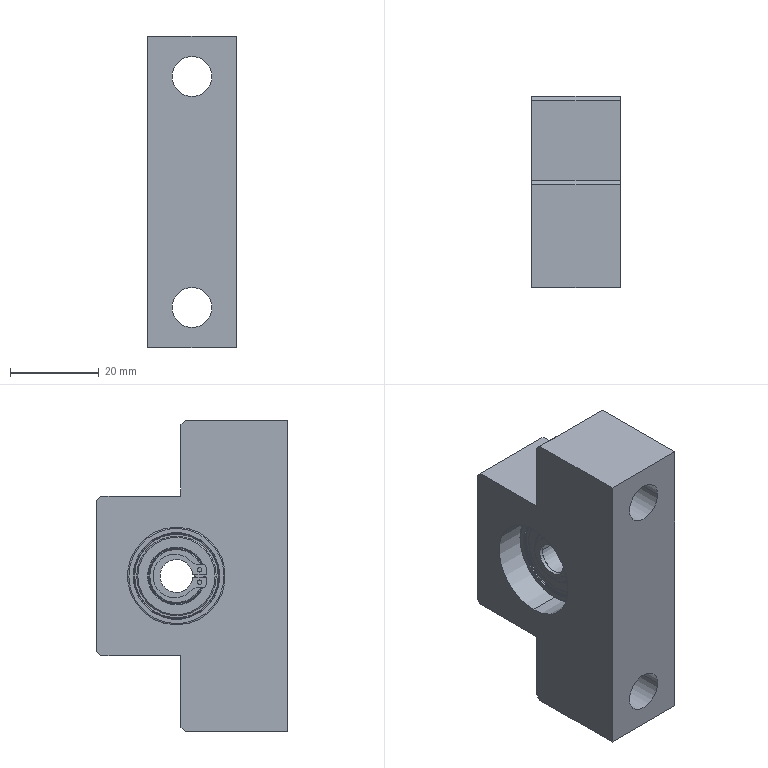Part | SolidWorks | 3 solids | 158 faces | box 20 x 43 x 70 mm | volume 38437 mm3 | cylinder 48 | cone 44 | plane 34 | spline 32 | commonest cylinder face diameters 1 x4 9 x4 12.2 x4 12.6 x4 12.73 x4 12.996 x4